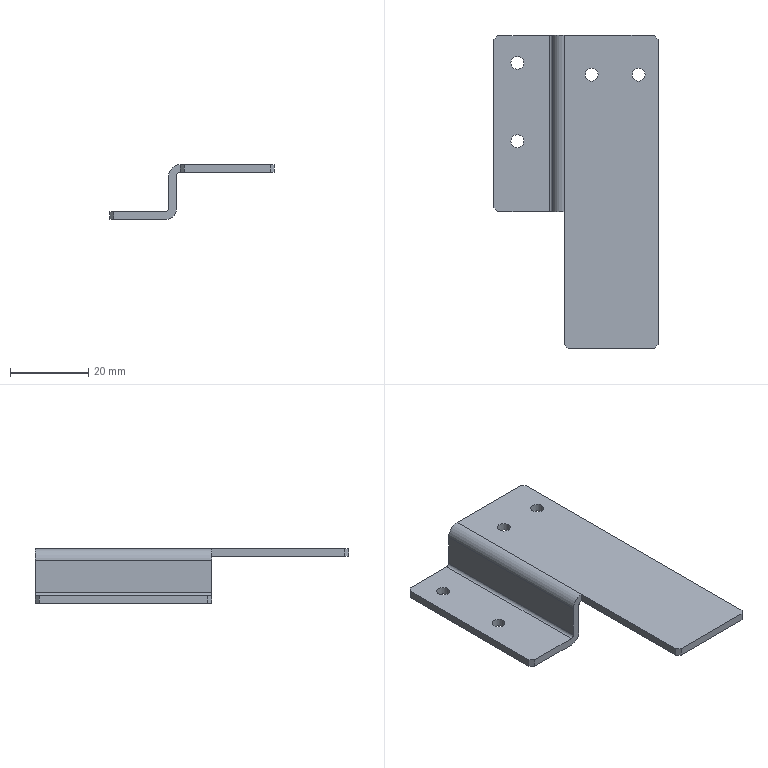Part | NX | 1 solid | 29 faces | box 42 x 80 x 14 mm | volume 6322 mm3 | plane 21 | cylinder 8 | commonest cylinder face diameters 3.3 x4 1.473 x1 2 x1 5.473 x1 6 x1
STEP:
#1=CARTESIAN_POINT('',(-14.5,-5.,-3.));
#2=VERTEX_POINT('',#1);
#3=CARTESIAN_POINT('',(-14.5,-5.,-11.263));
#4=VERTEX_POINT('',#3);
#5=CARTESIAN_POINT('',(-14.5,-5.,0.));
#6=DIRECTION('',(0.,0.,-1.));
#7=VECTOR('',#6,1000.);
#8=LINE('',#5,#7);
#9=EDGE_CURVE('',#2,#4,#8,.T.);
#10=ORIENTED_EDGE('',*,*,#9,.F.);
#11=CARTESIAN_POINT('',(-14.5,40.,-3.));
#12=VERTEX_POINT('',#11);
#13=CARTESIAN_POINT('',(-14.5,0.,-3.));
#14=DIRECTION('',(0.,1.,0.));
#15=VECTOR('',#14,1000.);
#16=LINE('',#13,#15);
#17=EDGE_CURVE('',#2,#12,#16,.T.);
#18=ORIENTED_EDGE('',*,*,#17,.T.);
#19=CARTESIAN_POINT('',(-14.5,40.,-11.263));
#20=VERTEX_POINT('',#19);
#21=CARTESIAN_POINT('',(-14.5,40.,-2.));
#22=DIRECTION('',(0.,0.,1.));
#23=VECTOR('',#22,1000.);
#24=LINE('',#21,#23);
#25=EDGE_CURVE('',#20,#12,#24,.T.);
#26=ORIENTED_EDGE('',*,*,#25,.F.);
#27=CARTESIAN_POINT('',(-14.5,-40.,-11.263));
#28=DIRECTION('',(0.,-1.,0.));
#29=VECTOR('',#28,1000.);
#30=LINE('',#27,#29);
#31=EDGE_CURVE('',#4,#20,#30,.F.);
#32=ORIENTED_EDGE('',*,*,#31,.F.);
#33=EDGE_LOOP('',(#10,#18,#26,#32));
#34=FACE_BOUND('',#33,.T.);
#35=CARTESIAN_POINT('',(-14.5,0.,0.));
#36=DIRECTION('',(-1.,0.,0.));
#37=DIRECTION('',(0.,0.,1.));
#38=AXIS2_PLACEMENT_3D('',#35,#36,#37);
#39=PLANE('',#38);
#40=ADVANCED_FACE('',(#34),#39,.T.);
#41=CARTESIAN_POINT('',(-12.5,-5.,-3.));
#42=VERTEX_POINT('',#41);
#43=CARTESIAN_POINT('',(-12.5,40.,-3.));
#44=VERTEX_POINT('',#43);
#45=CARTESIAN_POINT('',(-12.5,-40.,-3.));
#46=DIRECTION('',(0.,1.,0.));
#47=VECTOR('',#46,1000.);
#48=LINE('',#45,#47);
#49=EDGE_CURVE('',#42,#44,#48,.T.);
#50=ORIENTED_EDGE('',*,*,#49,.F.);
#51=CARTESIAN_POINT('',(-12.5,-5.,-11.263));
#52=VERTEX_POINT('',#51);
#53=CARTESIAN_POINT('',(-12.5,-5.,0.));
#54=DIRECTION('',(0.,0.,-1.));
#55=VECTOR('',#54,1000.);
#56=LINE('',#53,#55);
#57=EDGE_CURVE('',#42,#52,#56,.T.);
#58=ORIENTED_EDGE('',*,*,#57,.T.);
#59=CARTESIAN_POINT('',(-12.5,40.,-11.263));
#60=VERTEX_POINT('',#59);
#61=CARTESIAN_POINT('',(-12.5,-40.,-11.263));
#62=DIRECTION('',(0.,-1.,0.));
#63=VECTOR('',#62,1000.);
#64=LINE('',#61,#63);
#65=EDGE_CURVE('',#52,#60,#64,.F.);
#66=ORIENTED_EDGE('',*,*,#65,.T.);
#67=CARTESIAN_POINT('',(-12.5,40.,-2.));
#68=DIRECTION('',(0.,0.,1.));
#69=VECTOR('',#68,1000.);
#70=LINE('',#67,#69);
#71=EDGE_CURVE('',#60,#44,#70,.T.);
#72=ORIENTED_EDGE('',*,*,#71,.T.);
#73=EDGE_LOOP('',(#50,#58,#66,#72));
#74=FACE_BOUND('',#73,.T.);
#75=CARTESIAN_POINT('',(-12.5,0.,0.));
#76=DIRECTION('',(-1.,0.,0.));
#77=DIRECTION('',(0.,0.,1.));
#78=AXIS2_PLACEMENT_3D('',#75,#76,#77);
#79=PLANE('',#78);
#80=ADVANCED_FACE('',(#74),#79,.F.);
#81=CARTESIAN_POINT('',(11.5,40.,0.));
#82=VERTEX_POINT('',#81);
#83=CARTESIAN_POINT('',(-11.5,40.,0.));
#84=VERTEX_POINT('',#83);
#85=CARTESIAN_POINT('',(-12.5,40.,0.));
#86=DIRECTION('',(-1.,0.,0.));
#87=VECTOR('',#86,1000.);
#88=LINE('',#85,#87);
#89=EDGE_CURVE('',#82,#84,#88,.T.);
#90=ORIENTED_EDGE('',*,*,#89,.F.);
#91=CARTESIAN_POINT('',(11.5,40.,-2.));
#92=VERTEX_POINT('',#91);
#93=CARTESIAN_POINT('',(11.5,40.,-2.));
#94=DIRECTION('',(0.,0.,-1.));
#95=VECTOR('',#94,1000.);
#96=LINE('',#93,#95);
#97=EDGE_CURVE('',#82,#92,#96,.T.);
#98=ORIENTED_EDGE('',*,*,#97,.T.);
#99=CARTESIAN_POINT('',(-11.5,40.,-2.));
#100=VERTEX_POINT('',#99);
#101=CARTESIAN_POINT('',(-12.5,40.,-2.));
#102=DIRECTION('',(-1.,0.,0.));
#103=VECTOR('',#102,1000.);
#104=LINE('',#101,#103);
#105=EDGE_CURVE('',#92,#100,#104,.T.);
#106=ORIENTED_EDGE('',*,*,#105,.T.);
#107=CARTESIAN_POINT('',(-11.5,40.,-2.));
#108=DIRECTION('',(0.,0.,1.));
#109=VECTOR('',#108,1000.);
#110=LINE('',#107,#109);
#111=EDGE_CURVE('',#100,#84,#110,.T.);
#112=ORIENTED_EDGE('',*,*,#111,.T.);
#113=EDGE_LOOP('',(#90,#98,#106,#112));
#114=FACE_BOUND('',#113,.T.);
#115=CARTESIAN_POINT('',(-12.5,40.,-2.));
#116=DIRECTION('',(0.,1.,0.));
#117=DIRECTION('',(0.,0.,1.));
#118=AXIS2_PLACEMENT_3D('',#115,#116,#117);
#119=PLANE('',#118);
#120=ADVANCED_FACE('',(#114),#119,.T.);
#121=CARTESIAN_POINT('',(-2.85,30.,-2.));
#122=VERTEX_POINT('',#121);
#123=CARTESIAN_POINT('',(-4.5,30.,-2.));
#124=DIRECTION('',(0.,0.,1.));
#125=DIRECTION('',(1.,0.,0.));
#126=AXIS2_PLACEMENT_3D('',#123,#124,#125);
#127=CIRCLE('',#126,1.65);
#128=EDGE_CURVE('',#122,#122,#127,.T.);
#129=ORIENTED_EDGE('',*,*,#128,.T.);
#130=EDGE_LOOP('',(#129));
#131=FACE_BOUND('',#130,.T.);
#132=CARTESIAN_POINT('',(9.15,30.,-2.));
#133=VERTEX_POINT('',#132);
#134=CARTESIAN_POINT('',(7.5,30.,-2.));
#135=DIRECTION('',(0.,0.,1.));
#136=DIRECTION('',(1.,0.,0.));
#137=AXIS2_PLACEMENT_3D('',#134,#135,#136);
#138=CIRCLE('',#137,1.65);
#139=EDGE_CURVE('',#133,#133,#138,.T.);
#140=ORIENTED_EDGE('',*,*,#139,.T.);
#141=EDGE_LOOP('',(#140));
#142=FACE_BOUND('',#141,.T.);
#143=CARTESIAN_POINT('',(-10.5,-40.,-2.));
#144=VERTEX_POINT('',#143);
#145=CARTESIAN_POINT('',(11.5,-40.,-2.));
#146=VERTEX_POINT('',#145);
#147=CARTESIAN_POINT('',(-12.5,-40.,-2.));
#148=DIRECTION('',(1.,0.,0.));
#149=VECTOR('',#148,1000.);
#150=LINE('',#147,#149);
#151=EDGE_CURVE('',#144,#146,#150,.T.);
#152=ORIENTED_EDGE('',*,*,#151,.F.);
#153=CARTESIAN_POINT('',(-11.5,-39.,-2.));
#154=VERTEX_POINT('',#153);
#155=CARTESIAN_POINT('',(-25.25,-25.25,-2.));
#156=DIRECTION('',(-0.7071,0.7071,0.));
#157=VECTOR('',#156,1000.);
#158=LINE('',#155,#157);
#159=EDGE_CURVE('',#144,#154,#158,.T.);
#160=ORIENTED_EDGE('',*,*,#159,.T.);
#161=CARTESIAN_POINT('',(-11.5,-5.,-2.));
#162=VERTEX_POINT('',#161);
#163=CARTESIAN_POINT('',(-11.5,40.,-2.));
#164=DIRECTION('',(0.,1.,0.));
#165=VECTOR('',#164,1000.);
#166=LINE('',#163,#165);
#167=EDGE_CURVE('',#162,#154,#166,.F.);
#168=ORIENTED_EDGE('',*,*,#167,.F.);
#169=CARTESIAN_POINT('',(-11.5,40.,-2.));
#170=DIRECTION('',(0.,1.,0.));
#171=VECTOR('',#170,1000.);
#172=LINE('',#169,#171);
#173=EDGE_CURVE('',#100,#162,#172,.F.);
#174=ORIENTED_EDGE('',*,*,#173,.F.);
#175=ORIENTED_EDGE('',*,*,#105,.F.);
#176=CARTESIAN_POINT('',(12.5,39.,-2.));
#177=VERTEX_POINT('',#176);
#178=CARTESIAN_POINT('',(25.75,25.75,-2.));
#179=DIRECTION('',(-0.7071,0.7071,0.));
#180=VECTOR('',#179,1000.);
#181=LINE('',#178,#180);
#182=EDGE_CURVE('',#92,#177,#181,.F.);
#183=ORIENTED_EDGE('',*,*,#182,.T.);
#184=CARTESIAN_POINT('',(12.5,-39.,-2.));
#185=VERTEX_POINT('',#184);
#186=CARTESIAN_POINT('',(12.5,-40.,-2.));
#187=DIRECTION('',(0.,1.,0.));
#188=VECTOR('',#187,1000.);
#189=LINE('',#186,#188);
#190=EDGE_CURVE('',#185,#177,#189,.T.);
#191=ORIENTED_EDGE('',*,*,#190,.F.);
#192=CARTESIAN_POINT('',(25.75,-25.75,-2.));
#193=DIRECTION('',(0.7071,0.7071,0.));
#194=VECTOR('',#193,1000.);
#195=LINE('',#192,#194);
#196=EDGE_CURVE('',#185,#146,#195,.F.);
#197=ORIENTED_EDGE('',*,*,#196,.T.);
#198=EDGE_LOOP('',(#152,#160,#168,#174,#175,#183,#191,#197));
#199=FACE_BOUND('',#198,.T.);
#200=CARTESIAN_POINT('',(0.,0.,-2.));
#201=DIRECTION('',(0.,0.,-1.));
#202=DIRECTION('',(-1.,0.,0.));
#203=AXIS2_PLACEMENT_3D('',#200,#201,#202);
#204=PLANE('',#203);
#205=ADVANCED_FACE('',(#131,#142,#199),#204,.T.);
#206=CARTESIAN_POINT('',(-2.85,30.,0.));
#207=VERTEX_POINT('',#206);
#208=CARTESIAN_POINT('',(-4.5,30.,0.));
#209=DIRECTION('',(0.,0.,1.));
#210=DIRECTION('',(1.,0.,0.));
#211=AXIS2_PLACEMENT_3D('',#208,#209,#210);
#212=CIRCLE('',#211,1.65);
#213=EDGE_CURVE('',#207,#207,#212,.T.);
#214=ORIENTED_EDGE('',*,*,#213,.F.);
#215=EDGE_LOOP('',(#214));
#216=FACE_BOUND('',#215,.T.);
#217=CARTESIAN_POINT('',(9.15,30.,0.));
#218=VERTEX_POINT('',#217);
#219=CARTESIAN_POINT('',(7.5,30.,0.));
#220=DIRECTION('',(0.,0.,1.));
#221=DIRECTION('',(1.,0.,0.));
#222=AXIS2_PLACEMENT_3D('',#219,#220,#221);
#223=CIRCLE('',#222,1.65);
#224=EDGE_CURVE('',#218,#218,#223,.T.);
#225=ORIENTED_EDGE('',*,*,#224,.F.);
#226=EDGE_LOOP('',(#225));
#227=FACE_BOUND('',#226,.T.);
#228=CARTESIAN_POINT('',(-11.5,-5.,0.));
#229=VERTEX_POINT('',#228);
#230=CARTESIAN_POINT('',(-11.5,-39.,0.));
#231=VERTEX_POINT('',#230);
#232=CARTESIAN_POINT('',(-11.5,-5.,0.));
#233=DIRECTION('',(0.,-1.,0.));
#234=VECTOR('',#233,1000.);
#235=LINE('',#232,#234);
#236=EDGE_CURVE('',#229,#231,#235,.T.);
#237=ORIENTED_EDGE('',*,*,#236,.T.);
#238=CARTESIAN_POINT('',(-10.5,-40.,0.));
#239=VERTEX_POINT('',#238);
#240=CARTESIAN_POINT('',(-11.5,-39.,0.));
#241=DIRECTION('',(0.7071,-0.7071,0.));
#242=VECTOR('',#241,1000.);
#243=LINE('',#240,#242);
#244=EDGE_CURVE('',#231,#239,#243,.T.);
#245=ORIENTED_EDGE('',*,*,#244,.T.);
#246=CARTESIAN_POINT('',(11.5,-40.,0.));
#247=VERTEX_POINT('',#246);
#248=CARTESIAN_POINT('',(-12.5,-40.,0.));
#249=DIRECTION('',(1.,0.,0.));
#250=VECTOR('',#249,1000.);
#251=LINE('',#248,#250);
#252=EDGE_CURVE('',#239,#247,#251,.T.);
#253=ORIENTED_EDGE('',*,*,#252,.T.);
#254=CARTESIAN_POINT('',(12.5,-39.,0.));
#255=VERTEX_POINT('',#254);
#256=CARTESIAN_POINT('',(11.5,-40.,0.));
#257=DIRECTION('',(-0.7071,-0.7071,0.));
#258=VECTOR('',#257,1000.);
#259=LINE('',#256,#258);
#260=EDGE_CURVE('',#247,#255,#259,.F.);
#261=ORIENTED_EDGE('',*,*,#260,.T.);
#262=CARTESIAN_POINT('',(12.5,39.,0.));
#263=VERTEX_POINT('',#262);
#264=CARTESIAN_POINT('',(12.5,-40.,0.));
#265=DIRECTION('',(0.,1.,0.));
#266=VECTOR('',#265,1000.);
#267=LINE('',#264,#266);
#268=EDGE_CURVE('',#255,#263,#267,.T.);
#269=ORIENTED_EDGE('',*,*,#268,.T.);
#270=CARTESIAN_POINT('',(12.5,39.,0.));
#271=DIRECTION('',(0.7071,-0.7071,0.));
#272=VECTOR('',#271,1000.);
#273=LINE('',#270,#272);
#274=EDGE_CURVE('',#263,#82,#273,.F.);
#275=ORIENTED_EDGE('',*,*,#274,.T.);
#276=ORIENTED_EDGE('',*,*,#89,.T.);
#277=CARTESIAN_POINT('',(-11.5,40.,0.));
#278=DIRECTION('',(0.,1.,0.));
#279=VECTOR('',#278,1000.);
#280=LINE('',#277,#279);
#281=EDGE_CURVE('',#84,#229,#280,.F.);
#282=ORIENTED_EDGE('',*,*,#281,.T.);
#283=EDGE_LOOP('',(#237,#245,#253,#261,#269,#275,#276,#282));
#284=FACE_BOUND('',#283,.T.);
#285=CARTESIAN_POINT('',(0.,0.,0.));
#286=DIRECTION('',(0.,0.,-1.));
#287=DIRECTION('',(-1.,0.,0.));
#288=AXIS2_PLACEMENT_3D('',#285,#286,#287);
#289=PLANE('',#288);
#290=ADVANCED_FACE('',(#216,#227,#284),#289,.F.);
#291=ORIENTED_EDGE('',*,*,#268,.F.);
#292=CARTESIAN_POINT('',(12.5,-39.,-2.));
#293=DIRECTION('',(0.,0.,-1.));
#294=VECTOR('',#293,1000.);
#295=LINE('',#292,#294);
#296=EDGE_CURVE('',#255,#185,#295,.T.);
#297=ORIENTED_EDGE('',*,*,#296,.T.);
#298=ORIENTED_EDGE('',*,*,#190,.T.);
#299=CARTESIAN_POINT('',(12.5,39.,-2.));
#300=DIRECTION('',(0.,0.,1.));
#301=VECTOR('',#300,1000.);
#302=LINE('',#299,#301);
#303=EDGE_CURVE('',#177,#263,#302,.T.);
#304=ORIENTED_EDGE('',*,*,#303,.T.);
#305=EDGE_LOOP('',(#291,#297,#298,#304));
#306=FACE_BOUND('',#305,.T.);
#307=CARTESIAN_POINT('',(12.5,-40.,-2.));
#308=DIRECTION('',(1.,0.,0.));
#309=DIRECTION('',(0.,0.,-1.));
#310=AXIS2_PLACEMENT_3D('',#307,#308,#309);
#311=PLANE('',#310);
#312=ADVANCED_FACE('',(#306),#311,.T.);
#313=ORIENTED_EDGE('',*,*,#252,.F.);
#314=CARTESIAN_POINT('',(-10.5,-40.,-2.));
#315=DIRECTION('',(0.,0.,-1.));
#316=VECTOR('',#315,1000.);
#317=LINE('',#314,#316);
#318=EDGE_CURVE('',#239,#144,#317,.T.);
#319=ORIENTED_EDGE('',*,*,#318,.T.);
#320=ORIENTED_EDGE('',*,*,#151,.T.);
#321=CARTESIAN_POINT('',(11.5,-40.,-2.));
#322=DIRECTION('',(0.,0.,1.));
#323=VECTOR('',#322,1000.);
#324=LINE('',#321,#323);
#325=EDGE_CURVE('',#146,#247,#324,.T.);
#326=ORIENTED_EDGE('',*,*,#325,.T.);
#327=EDGE_LOOP('',(#313,#319,#320,#326));
#328=FACE_BOUND('',#327,.T.);
#329=CARTESIAN_POINT('',(-12.5,-40.,-2.));
#330=DIRECTION('',(0.,-1.,0.));
#331=DIRECTION('',(0.,0.,-1.));
#332=AXIS2_PLACEMENT_3D('',#329,#330,#331);
#333=PLANE('',#332);
#334=ADVANCED_FACE('',(#328),#333,.T.);
#335=ORIENTED_EDGE('',*,*,#128,.F.);
#336=EDGE_LOOP('',(#335));
#337=FACE_BOUND('',#336,.T.);
#338=ORIENTED_EDGE('',*,*,#213,.T.);
#339=EDGE_LOOP('',(#338));
#340=FACE_BOUND('',#339,.T.);
#341=CARTESIAN_POINT('',(-4.5,30.,0.));
#342=DIRECTION('',(0.,0.,1.));
#343=DIRECTION('',(1.,0.,0.));
#344=AXIS2_PLACEMENT_3D('',#341,#342,#343);
#345=CYLINDRICAL_SURFACE('',#344,1.65);
#346=ADVANCED_FACE('',(#337,#340),#345,.F.);
#347=ORIENTED_EDGE('',*,*,#139,.F.);
#348=EDGE_LOOP('',(#347));
#349=FACE_BOUND('',#348,.T.);
#350=ORIENTED_EDGE('',*,*,#224,.T.);
#351=EDGE_LOOP('',(#350));
#352=FACE_BOUND('',#351,.T.);
#353=CARTESIAN_POINT('',(7.5,30.,0.));
#354=DIRECTION('',(0.,0.,1.));
#355=DIRECTION('',(1.,0.,0.));
#356=AXIS2_PLACEMENT_3D('',#353,#354,#355);
#357=CYLINDRICAL_SURFACE('',#356,1.65);
#358=ADVANCED_FACE('',(#349,#352),#357,.F.);
#359=CARTESIAN_POINT('',(-11.5,40.,-3.));
#360=DIRECTION('',(0.,1.,0.));
#361=DIRECTION('',(0.,0.,1.));
#362=AXIS2_PLACEMENT_3D('',#359,#360,#361);
#363=CIRCLE('',#362,1.);
#364=EDGE_CURVE('',#44,#100,#363,.T.);
#365=ORIENTED_EDGE('',*,*,#364,.F.);
#366=CARTESIAN_POINT('',(-12.5,40.,-3.));
#367=DIRECTION('',(-1.,0.,0.));
#368=VECTOR('',#367,1000.);
#369=LINE('',#366,#368);
#370=EDGE_CURVE('',#44,#12,#369,.T.);
#371=ORIENTED_EDGE('',*,*,#370,.T.);
#372=CARTESIAN_POINT('',(-11.5,40.,-3.));
#373=DIRECTION('',(0.,1.,0.));
#374=DIRECTION('',(0.,0.,1.));
#375=AXIS2_PLACEMENT_3D('',#372,#373,#374);
#376=CIRCLE('',#375,3.);
#377=EDGE_CURVE('',#12,#84,#376,.T.);
#378=ORIENTED_EDGE('',*,*,#377,.T.);
#379=ORIENTED_EDGE('',*,*,#111,.F.);
#380=EDGE_LOOP('',(#365,#371,#378,#379));
#381=FACE_BOUND('',#380,.T.);
#382=CARTESIAN_POINT('',(-11.5,40.,-3.));
#383=DIRECTION('',(0.,-1.,0.));
#384=DIRECTION('',(0.,0.,-1.));
#385=AXIS2_PLACEMENT_3D('',#382,#383,#384);
#386=PLANE('',#385);
#387=ADVANCED_FACE('',(#381),#386,.F.);
#388=CARTESIAN_POINT('',(-11.5,-5.,-3.));
#389=DIRECTION('',(0.,1.,0.));
#390=DIRECTION('',(0.,0.,1.));
#391=AXIS2_PLACEMENT_3D('',#388,#389,#390);
#392=CIRCLE('',#391,3.);
#393=EDGE_CURVE('',#229,#2,#392,.F.);
#394=ORIENTED_EDGE('',*,*,#393,.F.);
#395=ORIENTED_EDGE('',*,*,#281,.F.);
#396=ORIENTED_EDGE('',*,*,#377,.F.);
#397=ORIENTED_EDGE('',*,*,#17,.F.);
#398=EDGE_LOOP('',(#394,#395,#396,#397));
#399=FACE_BOUND('',#398,.T.);
#400=CARTESIAN_POINT('',(-11.5,40.,-3.));
#401=DIRECTION('',(0.,1.,0.));
#402=DIRECTION('',(-1.,0.,0.));
#403=AXIS2_PLACEMENT_3D('',#400,#401,#402);
#404=CYLINDRICAL_SURFACE('',#403,3.);
#405=ADVANCED_FACE('',(#399),#404,.T.);
#406=ORIENTED_EDGE('',*,*,#173,.T.);
#407=CARTESIAN_POINT('',(-11.5,-5.,-3.));
#408=DIRECTION('',(0.,1.,0.));
#409=DIRECTION('',(0.,0.,1.));
#410=AXIS2_PLACEMENT_3D('',#407,#408,#409);
#411=CIRCLE('',#410,1.);
#412=EDGE_CURVE('',#162,#42,#411,.F.);
#413=ORIENTED_EDGE('',*,*,#412,.T.);
#414=ORIENTED_EDGE('',*,*,#49,.T.);
#415=ORIENTED_EDGE('',*,*,#364,.T.);
#416=EDGE_LOOP('',(#406,#413,#414,#415));
#417=FACE_BOUND('',#416,.T.);
#418=CARTESIAN_POINT('',(-11.5,40.,-3.));
#419=DIRECTION('',(0.,1.,0.));
#420=DIRECTION('',(-1.,0.,0.));
#421=AXIS2_PLACEMENT_3D('',#418,#419,#420);
#422=CYLINDRICAL_SURFACE('',#421,1.);
#423=ADVANCED_FACE('',(#417),#422,.F.);
#424=CARTESIAN_POINT('',(-14.5,40.,-11.263));
#425=DIRECTION('',(1.,0.,0.));
#426=VECTOR('',#425,1000.);
#427=LINE('',#424,#426);
#428=EDGE_CURVE('',#20,#60,#427,.T.);
#429=ORIENTED_EDGE('',*,*,#428,.F.);
#430=ORIENTED_EDGE('',*,*,#25,.T.);
#431=ORIENTED_EDGE('',*,*,#370,.F.);
#432=ORIENTED_EDGE('',*,*,#71,.F.);
#433=EDGE_LOOP('',(#429,#430,#431,#432));
#434=FACE_BOUND('',#433,.T.);
#435=CARTESIAN_POINT('',(-14.5,40.,-2.));
#436=DIRECTION('',(0.,1.,0.));
#437=DIRECTION('',(0.,0.,1.));
#438=AXIS2_PLACEMENT_3D('',#435,#436,#437);
#439=PLANE('',#438);
#440=ADVANCED_FACE('',(#434),#439,.T.);
#441=CARTESIAN_POINT('',(-15.237,40.,-12.));
#442=VERTEX_POINT('',#441);
#443=CARTESIAN_POINT('',(-15.237,40.,-14.));
#444=VERTEX_POINT('',#443);
#445=CARTESIAN_POINT('',(-15.237,40.,-12.));
#446=DIRECTION('',(0.,0.,-1.));
#447=VECTOR('',#446,1000.);
#448=LINE('',#445,#447);
#449=EDGE_CURVE('',#442,#444,#448,.T.);
#450=ORIENTED_EDGE('',*,*,#449,.F.);
#451=CARTESIAN_POINT('',(-15.237,40.,-11.263));
#452=DIRECTION('',(0.,-1.,0.));
#453=DIRECTION('',(0.,0.,-1.));
#454=AXIS2_PLACEMENT_3D('',#451,#452,#453);
#455=CIRCLE('',#454,0.7366);
#456=EDGE_CURVE('',#20,#442,#455,.F.);
#457=ORIENTED_EDGE('',*,*,#456,.F.);
#458=ORIENTED_EDGE('',*,*,#428,.T.);
#459=CARTESIAN_POINT('',(-15.237,40.,-11.263));
#460=DIRECTION('',(0.,-1.,0.));
#461=DIRECTION('',(0.,0.,-1.));
#462=AXIS2_PLACEMENT_3D('',#459,#460,#461);
#463=CIRCLE('',#462,2.737);
#464=EDGE_CURVE('',#60,#444,#463,.F.);
#465=ORIENTED_EDGE('',*,*,#464,.T.);
#466=EDGE_LOOP('',(#450,#457,#458,#465));
#467=FACE_BOUND('',#466,.T.);
#468=CARTESIAN_POINT('',(-15.237,40.,-11.263));
#469=DIRECTION('',(0.,1.,0.));
#470=DIRECTION('',(0.,0.,1.));
#471=AXIS2_PLACEMENT_3D('',#468,#469,#470);
#472=PLANE('',#471);
#473=ADVANCED_FACE('',(#467),#472,.T.);
#474=CARTESIAN_POINT('',(-15.237,-5.,-14.));
#475=VERTEX_POINT('',#474);
#476=CARTESIAN_POINT('',(-15.237,-5.,-11.263));
#477=DIRECTION('',(0.,1.,0.));
#478=DIRECTION('',(0.,0.,1.));
#479=AXIS2_PLACEMENT_3D('',#476,#477,#478);
#480=CIRCLE('',#479,2.737);
#481=EDGE_CURVE('',#475,#52,#480,.F.);
#482=ORIENTED_EDGE('',*,*,#481,.F.);
#483=CARTESIAN_POINT('',(-15.237,0.,-14.));
#484=DIRECTION('',(0.,-1.,0.));
#485=VECTOR('',#484,1000.);
#486=LINE('',#483,#485);
#487=EDGE_CURVE('',#444,#475,#486,.T.);
#488=ORIENTED_EDGE('',*,*,#487,.F.);
#489=ORIENTED_EDGE('',*,*,#464,.F.);
#490=ORIENTED_EDGE('',*,*,#65,.F.);
#491=EDGE_LOOP('',(#482,#488,#489,#490));
#492=FACE_BOUND('',#491,.T.);
#493=CARTESIAN_POINT('',(-15.237,-40.,-11.263));
#494=DIRECTION('',(0.,-1.,0.));
#495=DIRECTION('',(0.,0.,-1.));
#496=AXIS2_PLACEMENT_3D('',#493,#494,#495);
#497=CYLINDRICAL_SURFACE('',#496,2.737);
#498=ADVANCED_FACE('',(#492),#497,.T.);
#499=CARTESIAN_POINT('',(-15.237,-5.,-12.));
#500=VERTEX_POINT('',#499);
#501=CARTESIAN_POINT('',(-15.237,40.,-12.));
#502=DIRECTION('',(0.,-1.,0.));
#503=VECTOR('',#502,1000.);
#504=LINE('',#501,#503);
#505=EDGE_CURVE('',#442,#500,#504,.T.);
#506=ORIENTED_EDGE('',*,*,#505,.T.);
#507=CARTESIAN_POINT('',(-15.237,-5.,-11.263));
#508=DIRECTION('',(0.,1.,0.));
#509=DIRECTION('',(0.,0.,1.));
#510=AXIS2_PLACEMENT_3D('',#507,#508,#509);
#511=CIRCLE('',#510,0.7366);
#512=EDGE_CURVE('',#500,#4,#511,.F.);
#513=ORIENTED_EDGE('',*,*,#512,.T.);
#514=ORIENTED_EDGE('',*,*,#31,.T.);
#515=ORIENTED_EDGE('',*,*,#456,.T.);
#516=EDGE_LOOP('',(#506,#513,#514,#515));
#517=FACE_BOUND('',#516,.T.);
#518=CARTESIAN_POINT('',(-15.237,-40.,-11.263));
#519=DIRECTION('',(0.,-1.,0.));
#520=DIRECTION('',(0.,0.,-1.));
#521=AXIS2_PLACEMENT_3D('',#518,#519,#520);
#522=CYLINDRICAL_SURFACE('',#521,0.7366);
#523=ADVANCED_FACE('',(#517),#522,.F.);
#524=CARTESIAN_POINT('',(-28.5,40.,-14.));
#525=VERTEX_POINT('',#524);
#526=CARTESIAN_POINT('',(-29.5,40.,-14.));
#527=DIRECTION('',(-1.,0.,0.));
#528=VECTOR('',#527,1000.);
#529=LINE('',#526,#528);
#530=EDGE_CURVE('',#444,#525,#529,.T.);
#531=ORIENTED_EDGE('',*,*,#530,.T.);
#532=CARTESIAN_POINT('',(-28.5,40.,-12.));
#533=VERTEX_POINT('',#532);
#534=CARTESIAN_POINT('',(-28.5,40.,-14.));
#535=DIRECTION('',(0.,0.,1.));
#536=VECTOR('',#535,1000.);
#537=LINE('',#534,#536);
#538=EDGE_CURVE('',#525,#533,#537,.T.);
#539=ORIENTED_EDGE('',*,*,#538,.T.);
#540=CARTESIAN_POINT('',(-29.5,40.,-12.));
#541=DIRECTION('',(-1.,0.,0.));
#542=VECTOR('',#541,1000.);
#543=LINE('',#540,#542);
#544=EDGE_CURVE('',#442,#533,#543,.T.);
#545=ORIENTED_EDGE('',*,*,#544,.F.);
#546=ORIENTED_EDGE('',*,*,#449,.T.);
#547=EDGE_LOOP('',(#531,#539,#545,#546));
#548=FACE_BOUND('',#547,.T.);
#549=CARTESIAN_POINT('',(-29.5,40.,-14.));
#550=DIRECTION('',(0.,1.,0.));
#551=DIRECTION('',(-1.,0.,0.));
#552=AXIS2_PLACEMENT_3D('',#549,#550,#551);
#553=PLANE('',#552);
#554=ADVANCED_FACE('',(#548),#553,.T.);
#555=CARTESIAN_POINT('',(-28.5,-5.,-14.));
#556=VERTEX_POINT('',#555);
#557=CARTESIAN_POINT('',(-11.5,-5.,-14.));
#558=DIRECTION('',(1.,0.,0.));
#559=VECTOR('',#558,1000.);
#560=LINE('',#557,#559);
#561=EDGE_CURVE('',#556,#475,#560,.T.);
#562=ORIENTED_EDGE('',*,*,#561,.F.);
#563=CARTESIAN_POINT('',(-29.5,-4.,-14.));
#564=VERTEX_POINT('',#563);
#565=CARTESIAN_POINT('',(-16.75,-16.75,-14.));
#566=DIRECTION('',(-0.7071,0.7071,0.));
#567=VECTOR('',#566,1000.);
#568=LINE('',#565,#567);
#569=EDGE_CURVE('',#556,#564,#568,.T.);
#570=ORIENTED_EDGE('',*,*,#569,.T.);
#571=CARTESIAN_POINT('',(-29.5,39.,-14.));
#572=VERTEX_POINT('',#571);
#573=CARTESIAN_POINT('',(-29.5,-40.,-14.));
#574=DIRECTION('',(0.,-1.,0.));
#575=VECTOR('',#574,1000.);
#576=LINE('',#573,#575);
#577=EDGE_CURVE('',#572,#564,#576,.T.);
#578=ORIENTED_EDGE('',*,*,#577,.F.);
#579=CARTESIAN_POINT('',(-34.25,34.25,-14.));
#580=DIRECTION('',(-0.7071,-0.7071,0.));
#581=VECTOR('',#580,1000.);
#582=LINE('',#579,#581);
#583=EDGE_CURVE('',#572,#525,#582,.F.);
#584=ORIENTED_EDGE('',*,*,#583,.T.);
#585=ORIENTED_EDGE('',*,*,#530,.F.);
#586=ORIENTED_EDGE('',*,*,#487,.T.);
#587=EDGE_LOOP('',(#562,#570,#578,#584,#585,#586));
#588=FACE_BOUND('',#587,.T.);
#589=CARTESIAN_POINT('',(-25.15,33.,-14.));
#590=VERTEX_POINT('',#589);
#591=CARTESIAN_POINT('',(-23.5,33.,-14.));
#592=DIRECTION('',(0.,0.,-1.));
#593=DIRECTION('',(-1.,0.,0.));
#594=AXIS2_PLACEMENT_3D('',#591,#592,#593);
#595=CIRCLE('',#594,1.65);
#596=EDGE_CURVE('',#590,#590,#595,.T.);
#597=ORIENTED_EDGE('',*,*,#596,.F.);
#598=EDGE_LOOP('',(#597));
#599=FACE_BOUND('',#598,.T.);
#600=CARTESIAN_POINT('',(-25.15,13.,-14.));
#601=VERTEX_POINT('',#600);
#602=CARTESIAN_POINT('',(-23.5,13.,-14.));
#603=DIRECTION('',(0.,0.,-1.));
#604=DIRECTION('',(-1.,0.,0.));
#605=AXIS2_PLACEMENT_3D('',#602,#603,#604);
#606=CIRCLE('',#605,1.65);
#607=EDGE_CURVE('',#601,#601,#606,.T.);
#608=ORIENTED_EDGE('',*,*,#607,.F.);
#609=EDGE_LOOP('',(#608));
#610=FACE_BOUND('',#609,.T.);
#611=CARTESIAN_POINT('',(0.,0.,-14.));
#612=DIRECTION('',(0.,0.,-1.));
#613=DIRECTION('',(-1.,0.,0.));
#614=AXIS2_PLACEMENT_3D('',#611,#612,#613);
#615=PLANE('',#614);
#616=ADVANCED_FACE('',(#588,#599,#610),#615,.T.);
#617=CARTESIAN_POINT('',(-25.15,33.,-12.));
#618=VERTEX_POINT('',#617);
#619=CARTESIAN_POINT('',(-23.5,33.,-12.));
#620=DIRECTION('',(0.,0.,-1.));
#621=DIRECTION('',(-1.,0.,0.));
#622=AXIS2_PLACEMENT_3D('',#619,#620,#621);
#623=CIRCLE('',#622,1.65);
#624=EDGE_CURVE('',#618,#618,#623,.T.);
#625=ORIENTED_EDGE('',*,*,#624,.T.);
#626=EDGE_LOOP('',(#625));
#627=FACE_BOUND('',#626,.T.);
#628=CARTESIAN_POINT('',(-25.15,13.,-12.));
#629=VERTEX_POINT('',#628);
#630=CARTESIAN_POINT('',(-23.5,13.,-12.));
#631=DIRECTION('',(0.,0.,-1.));
#632=DIRECTION('',(-1.,0.,0.));
#633=AXIS2_PLACEMENT_3D('',#630,#631,#632);
#634=CIRCLE('',#633,1.65);
#635=EDGE_CURVE('',#629,#629,#634,.T.);
#636=ORIENTED_EDGE('',*,*,#635,.T.);
#637=EDGE_LOOP('',(#636));
#638=FACE_BOUND('',#637,.T.);
#639=CARTESIAN_POINT('',(-29.5,39.,-12.));
#640=VERTEX_POINT('',#639);
#641=CARTESIAN_POINT('',(-29.5,-4.,-12.));
#642=VERTEX_POINT('',#641);
#643=CARTESIAN_POINT('',(-29.5,-40.,-12.));
#644=DIRECTION('',(0.,-1.,0.));
#645=VECTOR('',#644,1000.);
#646=LINE('',#643,#645);
#647=EDGE_CURVE('',#640,#642,#646,.T.);
#648=ORIENTED_EDGE('',*,*,#647,.T.);
#649=CARTESIAN_POINT('',(-28.5,-5.,-12.));
#650=VERTEX_POINT('',#649);
#651=CARTESIAN_POINT('',(-28.5,-5.,-12.));
#652=DIRECTION('',(0.7071,-0.7071,0.));
#653=VECTOR('',#652,1000.);
#654=LINE('',#651,#653);
#655=EDGE_CURVE('',#642,#650,#654,.T.);
#656=ORIENTED_EDGE('',*,*,#655,.T.);
#657=CARTESIAN_POINT('',(0.,-5.,-12.));
#658=DIRECTION('',(1.,0.,0.));
#659=VECTOR('',#658,1000.);
#660=LINE('',#657,#659);
#661=EDGE_CURVE('',#650,#500,#660,.T.);
#662=ORIENTED_EDGE('',*,*,#661,.T.);
#663=ORIENTED_EDGE('',*,*,#505,.F.);
#664=ORIENTED_EDGE('',*,*,#544,.T.);
#665=CARTESIAN_POINT('',(-28.5,40.,-12.));
#666=DIRECTION('',(0.7071,0.7071,0.));
#667=VECTOR('',#666,1000.);
#668=LINE('',#665,#667);
#669=EDGE_CURVE('',#533,#640,#668,.F.);
#670=ORIENTED_EDGE('',*,*,#669,.T.);
#671=EDGE_LOOP('',(#648,#656,#662,#663,#664,#670));
#672=FACE_BOUND('',#671,.T.);
#673=CARTESIAN_POINT('',(0.,0.,-12.));
#674=DIRECTION('',(0.,0.,-1.));
#675=DIRECTION('',(-1.,0.,0.));
#676=AXIS2_PLACEMENT_3D('',#673,#674,#675);
#677=PLANE('',#676);
#678=ADVANCED_FACE('',(#627,#638,#672),#677,.F.);
#679=ORIENTED_EDGE('',*,*,#577,.T.);
#680=CARTESIAN_POINT('',(-29.5,-4.,-12.));
#681=DIRECTION('',(0.,0.,1.));
#682=VECTOR('',#681,1000.);
#683=LINE('',#680,#682);
#684=EDGE_CURVE('',#564,#642,#683,.T.);
#685=ORIENTED_EDGE('',*,*,#684,.T.);
#686=ORIENTED_EDGE('',*,*,#647,.F.);
#687=CARTESIAN_POINT('',(-29.5,39.,-14.));
#688=DIRECTION('',(0.,0.,-1.));
#689=VECTOR('',#688,1000.);
#690=LINE('',#687,#689);
#691=EDGE_CURVE('',#640,#572,#690,.T.);
#692=ORIENTED_EDGE('',*,*,#691,.T.);
#693=EDGE_LOOP('',(#679,#685,#686,#692));
#694=FACE_BOUND('',#693,.T.);
#695=CARTESIAN_POINT('',(-29.5,-40.,-14.));
#696=DIRECTION('',(-1.,0.,0.));
#697=DIRECTION('',(0.,0.,1.));
#698=AXIS2_PLACEMENT_3D('',#695,#696,#697);
#699=PLANE('',#698);
#700=ADVANCED_FACE('',(#694),#699,.T.);
#701=ORIENTED_EDGE('',*,*,#607,.T.);
#702=EDGE_LOOP('',(#701));
#703=FACE_BOUND('',#702,.T.);
#704=ORIENTED_EDGE('',*,*,#635,.F.);
#705=EDGE_LOOP('',(#704));
#706=FACE_BOUND('',#705,.T.);
#707=CARTESIAN_POINT('',(-23.5,13.,-14.));
#708=DIRECTION('',(0.,0.,-1.));
#709=DIRECTION('',(-1.,0.,0.));
#710=AXIS2_PLACEMENT_3D('',#707,#708,#709);
#711=CYLINDRICAL_SURFACE('',#710,1.65);
#712=ADVANCED_FACE('',(#703,#706),#711,.F.);
#713=ORIENTED_EDGE('',*,*,#596,.T.);
#714=EDGE_LOOP('',(#713));
#715=FACE_BOUND('',#714,.T.);
#716=ORIENTED_EDGE('',*,*,#624,.F.);
#717=EDGE_LOOP('',(#716));
#718=FACE_BOUND('',#717,.T.);
#719=CARTESIAN_POINT('',(-23.5,33.,-14.));
#720=DIRECTION('',(0.,0.,-1.));
#721=DIRECTION('',(-1.,0.,0.));
#722=AXIS2_PLACEMENT_3D('',#719,#720,#721);
#723=CYLINDRICAL_SURFACE('',#722,1.65);
#724=ADVANCED_FACE('',(#715,#718),#723,.F.);
#725=ORIENTED_EDGE('',*,*,#583,.F.);
#726=ORIENTED_EDGE('',*,*,#691,.F.);
#727=ORIENTED_EDGE('',*,*,#669,.F.);
#728=ORIENTED_EDGE('',*,*,#538,.F.);
#729=EDGE_LOOP('',(#725,#726,#727,#728));
#730=FACE_BOUND('',#729,.T.);
#731=CARTESIAN_POINT('',(-28.5,40.,-14.));
#732=DIRECTION('',(0.7071,-0.7071,0.));
#733=DIRECTION('',(0.,0.,1.));
#734=AXIS2_PLACEMENT_3D('',#731,#732,#733);
#735=PLANE('',#734);
#736=ADVANCED_FACE('',(#730),#735,.F.);
#737=ORIENTED_EDGE('',*,*,#196,.F.);
#738=ORIENTED_EDGE('',*,*,#296,.F.);
#739=ORIENTED_EDGE('',*,*,#260,.F.);
#740=ORIENTED_EDGE('',*,*,#325,.F.);
#741=EDGE_LOOP('',(#737,#738,#739,#740));
#742=FACE_BOUND('',#741,.T.);
#743=CARTESIAN_POINT('',(11.5,-40.,-2.));
#744=DIRECTION('',(-0.7071,0.7071,0.));
#745=DIRECTION('',(0.,0.,1.));
#746=AXIS2_PLACEMENT_3D('',#743,#744,#745);
#747=PLANE('',#746);
#748=ADVANCED_FACE('',(#742),#747,.F.);
#749=ORIENTED_EDGE('',*,*,#182,.F.);
#750=ORIENTED_EDGE('',*,*,#97,.F.);
#751=ORIENTED_EDGE('',*,*,#274,.F.);
#752=ORIENTED_EDGE('',*,*,#303,.F.);
#753=EDGE_LOOP('',(#749,#750,#751,#752));
#754=FACE_BOUND('',#753,.T.);
#755=CARTESIAN_POINT('',(12.5,39.,-2.));
#756=DIRECTION('',(-0.7071,-0.7071,0.));
#757=DIRECTION('',(0.,0.,1.));
#758=AXIS2_PLACEMENT_3D('',#755,#756,#757);
#759=PLANE('',#758);
#760=ADVANCED_FACE('',(#754),#759,.F.);
#761=ORIENTED_EDGE('',*,*,#167,.T.);
#762=CARTESIAN_POINT('',(-11.5,-39.,0.));
#763=DIRECTION('',(0.,0.,1.));
#764=VECTOR('',#763,1000.);
#765=LINE('',#762,#764);
#766=EDGE_CURVE('',#154,#231,#765,.T.);
#767=ORIENTED_EDGE('',*,*,#766,.T.);
#768=ORIENTED_EDGE('',*,*,#236,.F.);
#769=CARTESIAN_POINT('',(-11.5,-5.,0.));
#770=DIRECTION('',(0.,0.,1.));
#771=VECTOR('',#770,1000.);
#772=LINE('',#769,#771);
#773=EDGE_CURVE('',#162,#229,#772,.T.);
#774=ORIENTED_EDGE('',*,*,#773,.F.);
#775=EDGE_LOOP('',(#761,#767,#768,#774));
#776=FACE_BOUND('',#775,.T.);
#777=CARTESIAN_POINT('',(-11.5,-5.,0.));
#778=DIRECTION('',(1.,0.,0.));
#779=DIRECTION('',(0.,0.,-1.));
#780=AXIS2_PLACEMENT_3D('',#777,#778,#779);
#781=PLANE('',#780);
#782=ADVANCED_FACE('',(#776),#781,.F.);
#783=ORIENTED_EDGE('',*,*,#661,.F.);
#784=CARTESIAN_POINT('',(-28.5,-5.,-14.));
#785=DIRECTION('',(0.,0.,-1.));
#786=VECTOR('',#785,1000.);
#787=LINE('',#784,#786);
#788=EDGE_CURVE('',#650,#556,#787,.T.);
#789=ORIENTED_EDGE('',*,*,#788,.T.);
#790=ORIENTED_EDGE('',*,*,#561,.T.);
#791=ORIENTED_EDGE('',*,*,#481,.T.);
#792=ORIENTED_EDGE('',*,*,#57,.F.);
#793=ORIENTED_EDGE('',*,*,#412,.F.);
#794=ORIENTED_EDGE('',*,*,#773,.T.);
#795=ORIENTED_EDGE('',*,*,#393,.T.);
#796=ORIENTED_EDGE('',*,*,#9,.T.);
#797=ORIENTED_EDGE('',*,*,#512,.F.);
#798=EDGE_LOOP('',(#783,#789,#790,#791,#792,#793,#794,#795,#796,#797));
#799=FACE_BOUND('',#798,.T.);
#800=CARTESIAN_POINT('',(0.,-5.,0.));
#801=DIRECTION('',(0.,1.,0.));
#802=DIRECTION('',(0.,0.,1.));
#803=AXIS2_PLACEMENT_3D('',#800,#801,#802);
#804=PLANE('',#803);
#805=ADVANCED_FACE('',(#799),#804,.F.);
#806=ORIENTED_EDGE('',*,*,#159,.F.);
#807=ORIENTED_EDGE('',*,*,#318,.F.);
#808=ORIENTED_EDGE('',*,*,#244,.F.);
#809=ORIENTED_EDGE('',*,*,#766,.F.);
#810=EDGE_LOOP('',(#806,#807,#808,#809));
#811=FACE_BOUND('',#810,.T.);
#812=CARTESIAN_POINT('',(-11.5,-39.,0.));
#813=DIRECTION('',(-0.7071,-0.7071,0.));
#814=DIRECTION('',(0.,0.,-1.));
#815=AXIS2_PLACEMENT_3D('',#812,#813,#814);
#816=PLANE('',#815);
#817=ADVANCED_FACE('',(#811),#816,.T.);
#818=ORIENTED_EDGE('',*,*,#655,.F.);
#819=ORIENTED_EDGE('',*,*,#684,.F.);
#820=ORIENTED_EDGE('',*,*,#569,.F.);
#821=ORIENTED_EDGE('',*,*,#788,.F.);
#822=EDGE_LOOP('',(#818,#819,#820,#821));
#823=FACE_BOUND('',#822,.T.);
#824=CARTESIAN_POINT('',(-28.5,-5.,0.));
#825=DIRECTION('',(-0.7071,-0.7071,0.));
#826=DIRECTION('',(0.,0.,1.));
#827=AXIS2_PLACEMENT_3D('',#824,#825,#826);
#828=PLANE('',#827);
#829=ADVANCED_FACE('',(#823),#828,.T.);
#830=CLOSED_SHELL('',(#40,#80,#120,#205,#290,#312,#334,#346,#358,#387,#405,#423,#440,#473,#498,#523,#554,#616,#678,#700,#712,#724,#736,#748,#760,#782,#805,#817,#829));
#831=MANIFOLD_SOLID_BREP('',#830);
#832=(LENGTH_UNIT()NAMED_UNIT(*)SI_UNIT(.MILLI.,.METRE.));
#833=UNCERTAINTY_MEASURE_WITH_UNIT(LENGTH_MEASURE(0.00001),#832,'','');
#834=(NAMED_UNIT(*)PLANE_ANGLE_UNIT()SI_UNIT($,.RADIAN.));
#835=(NAMED_UNIT(*)SI_UNIT($,.STERADIAN.)SOLID_ANGLE_UNIT());
#836=(GEOMETRIC_REPRESENTATION_CONTEXT(3)GLOBAL_UNCERTAINTY_ASSIGNED_CONTEXT((#833))GLOBAL_UNIT_ASSIGNED_CONTEXT((#832,#834,#835))REPRESENTATION_CONTEXT('',''));
#837=ADVANCED_BREP_SHAPE_REPRESENTATION('',(#831),#836);